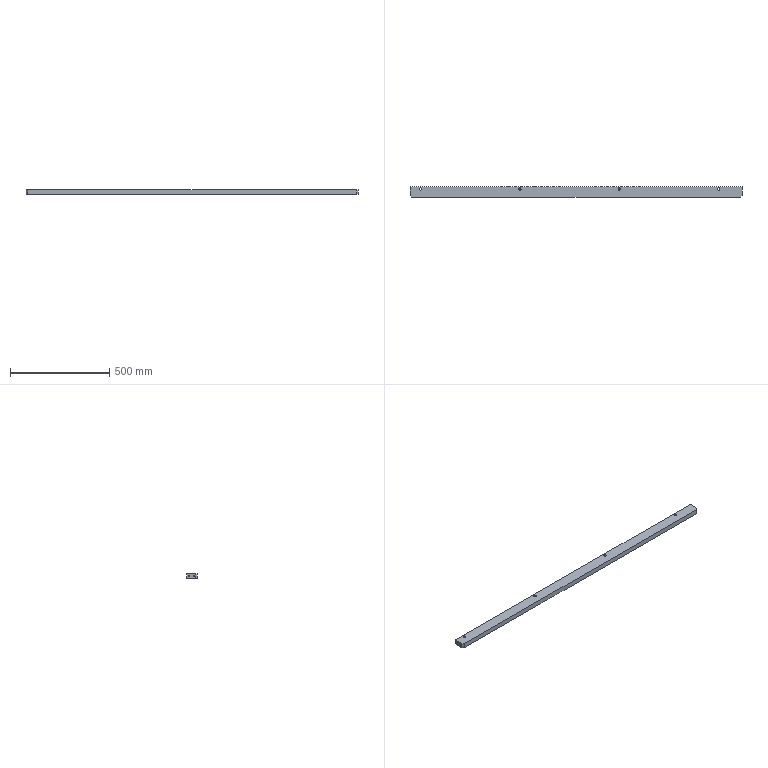Part | STEP file | J452-EBZ05-19-04-Part-1 | 1 solid | 30 faces | box 1670 x 55 x 25 mm | volume 2280219 mm3 | cylinder 16 | plane 10 | cone 4 | commonest cylinder face diameters 12 x8 6.9 x4 8 x4